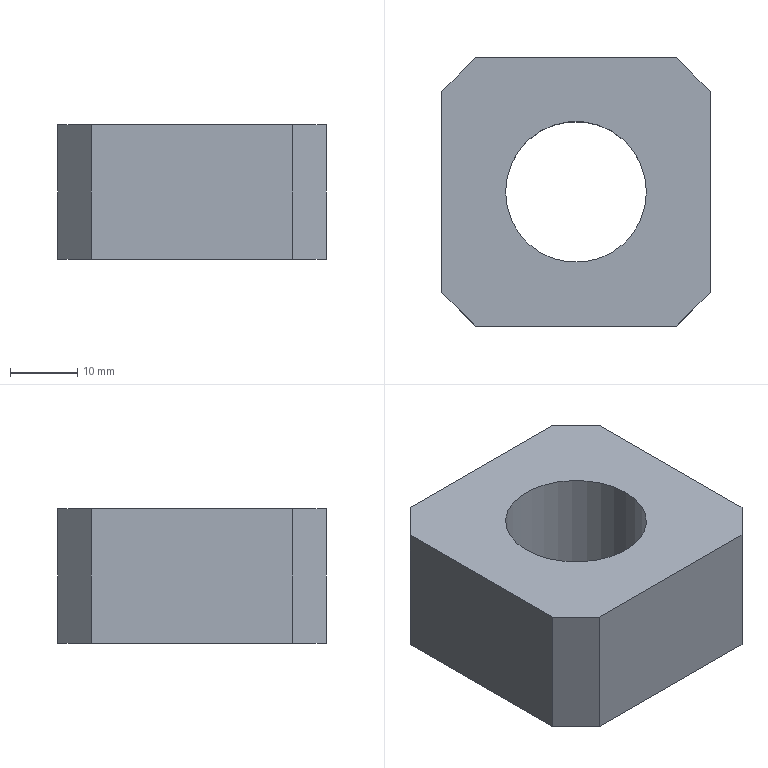Part | NX | 1 solid | 11 faces | box 40 x 40 x 20 mm | volume 24073 mm3 | plane 10 | cylinder 1 | commonest cylinder face diameters 21 x1
STEP:
#1=CARTESIAN_POINT('',(30.5,20.,20.));
#2=VERTEX_POINT('',#1);
#3=CARTESIAN_POINT('',(20.,20.,20.));
#4=DIRECTION('',(0.,0.,1.));
#5=DIRECTION('',(1.,0.,0.));
#6=AXIS2_PLACEMENT_3D('',#3,#4,#5);
#7=CIRCLE('',#6,10.5);
#8=EDGE_CURVE('',#2,#2,#7,.F.);
#9=ORIENTED_EDGE('',*,*,#8,.T.);
#10=EDGE_LOOP('',(#9));
#11=FACE_BOUND('',#10,.T.);
#12=CARTESIAN_POINT('',(35.,0.,20.));
#13=VERTEX_POINT('',#12);
#14=CARTESIAN_POINT('',(5.,0.,20.));
#15=VERTEX_POINT('',#14);
#16=CARTESIAN_POINT('',(20.,0.,20.));
#17=DIRECTION('',(-1.,0.,0.));
#18=VECTOR('',#17,1000.);
#19=LINE('',#16,#18);
#20=EDGE_CURVE('',#13,#15,#19,.T.);
#21=ORIENTED_EDGE('',*,*,#20,.F.);
#22=CARTESIAN_POINT('',(40.,5.,20.));
#23=VERTEX_POINT('',#22);
#24=CARTESIAN_POINT('',(37.5,2.5,20.));
#25=DIRECTION('',(-0.7071,-0.7071,0.));
#26=VECTOR('',#25,1000.);
#27=LINE('',#24,#26);
#28=EDGE_CURVE('',#13,#23,#27,.F.);
#29=ORIENTED_EDGE('',*,*,#28,.T.);
#30=CARTESIAN_POINT('',(40.,35.,20.));
#31=VERTEX_POINT('',#30);
#32=CARTESIAN_POINT('',(40.,20.,20.));
#33=DIRECTION('',(0.,-1.,0.));
#34=VECTOR('',#33,1000.);
#35=LINE('',#32,#34);
#36=EDGE_CURVE('',#31,#23,#35,.T.);
#37=ORIENTED_EDGE('',*,*,#36,.F.);
#38=CARTESIAN_POINT('',(35.,40.,20.));
#39=VERTEX_POINT('',#38);
#40=CARTESIAN_POINT('',(37.5,37.5,20.));
#41=DIRECTION('',(0.7071,-0.7071,0.));
#42=VECTOR('',#41,1000.);
#43=LINE('',#40,#42);
#44=EDGE_CURVE('',#31,#39,#43,.F.);
#45=ORIENTED_EDGE('',*,*,#44,.T.);
#46=CARTESIAN_POINT('',(5.,40.,20.));
#47=VERTEX_POINT('',#46);
#48=CARTESIAN_POINT('',(20.,40.,20.));
#49=DIRECTION('',(1.,0.,0.));
#50=VECTOR('',#49,1000.);
#51=LINE('',#48,#50);
#52=EDGE_CURVE('',#47,#39,#51,.T.);
#53=ORIENTED_EDGE('',*,*,#52,.F.);
#54=CARTESIAN_POINT('',(0.,35.,20.));
#55=VERTEX_POINT('',#54);
#56=CARTESIAN_POINT('',(2.5,37.5,20.));
#57=DIRECTION('',(0.7071,0.7071,0.));
#58=VECTOR('',#57,1000.);
#59=LINE('',#56,#58);
#60=EDGE_CURVE('',#47,#55,#59,.F.);
#61=ORIENTED_EDGE('',*,*,#60,.T.);
#62=CARTESIAN_POINT('',(0.,5.,20.));
#63=VERTEX_POINT('',#62);
#64=CARTESIAN_POINT('',(0.,20.,20.));
#65=DIRECTION('',(0.,1.,0.));
#66=VECTOR('',#65,1000.);
#67=LINE('',#64,#66);
#68=EDGE_CURVE('',#63,#55,#67,.T.);
#69=ORIENTED_EDGE('',*,*,#68,.F.);
#70=CARTESIAN_POINT('',(2.5,2.5,20.));
#71=DIRECTION('',(-0.7071,0.7071,0.));
#72=VECTOR('',#71,1000.);
#73=LINE('',#70,#72);
#74=EDGE_CURVE('',#63,#15,#73,.F.);
#75=ORIENTED_EDGE('',*,*,#74,.T.);
#76=EDGE_LOOP('',(#21,#29,#37,#45,#53,#61,#69,#75));
#77=FACE_BOUND('',#76,.T.);
#78=CARTESIAN_POINT('',(20.,20.,20.));
#79=DIRECTION('',(0.,0.,1.));
#80=DIRECTION('',(1.,0.,0.));
#81=AXIS2_PLACEMENT_3D('',#78,#79,#80);
#82=PLANE('',#81);
#83=ADVANCED_FACE('',(#11,#77),#82,.T.);
#84=CARTESIAN_POINT('',(5.,0.,0.));
#85=VERTEX_POINT('',#84);
#86=CARTESIAN_POINT('',(35.,0.,0.));
#87=VERTEX_POINT('',#86);
#88=CARTESIAN_POINT('',(20.,0.,0.));
#89=DIRECTION('',(1.,0.,0.));
#90=VECTOR('',#89,1000.);
#91=LINE('',#88,#90);
#92=EDGE_CURVE('',#85,#87,#91,.T.);
#93=ORIENTED_EDGE('',*,*,#92,.T.);
#94=CARTESIAN_POINT('',(35.,0.,0.));
#95=DIRECTION('',(0.,0.,1.));
#96=VECTOR('',#95,1000.);
#97=LINE('',#94,#96);
#98=EDGE_CURVE('',#87,#13,#97,.T.);
#99=ORIENTED_EDGE('',*,*,#98,.T.);
#100=ORIENTED_EDGE('',*,*,#20,.T.);
#101=CARTESIAN_POINT('',(5.,0.,0.));
#102=DIRECTION('',(0.,0.,-1.));
#103=VECTOR('',#102,1000.);
#104=LINE('',#101,#103);
#105=EDGE_CURVE('',#15,#85,#104,.T.);
#106=ORIENTED_EDGE('',*,*,#105,.T.);
#107=EDGE_LOOP('',(#93,#99,#100,#106));
#108=FACE_BOUND('',#107,.T.);
#109=CARTESIAN_POINT('',(20.,0.,0.));
#110=DIRECTION('',(0.,-1.,0.));
#111=DIRECTION('',(0.,0.,-1.));
#112=AXIS2_PLACEMENT_3D('',#109,#110,#111);
#113=PLANE('',#112);
#114=ADVANCED_FACE('',(#108),#113,.T.);
#115=ORIENTED_EDGE('',*,*,#68,.T.);
#116=CARTESIAN_POINT('',(0.,35.,0.));
#117=VERTEX_POINT('',#116);
#118=CARTESIAN_POINT('',(0.,35.,0.));
#119=DIRECTION('',(0.,0.,-1.));
#120=VECTOR('',#119,1000.);
#121=LINE('',#118,#120);
#122=EDGE_CURVE('',#55,#117,#121,.T.);
#123=ORIENTED_EDGE('',*,*,#122,.T.);
#124=CARTESIAN_POINT('',(0.,5.,0.));
#125=VERTEX_POINT('',#124);
#126=CARTESIAN_POINT('',(0.,20.,0.));
#127=DIRECTION('',(0.,-1.,0.));
#128=VECTOR('',#127,1000.);
#129=LINE('',#126,#128);
#130=EDGE_CURVE('',#117,#125,#129,.T.);
#131=ORIENTED_EDGE('',*,*,#130,.T.);
#132=CARTESIAN_POINT('',(0.,5.,0.));
#133=DIRECTION('',(0.,0.,1.));
#134=VECTOR('',#133,1000.);
#135=LINE('',#132,#134);
#136=EDGE_CURVE('',#125,#63,#135,.T.);
#137=ORIENTED_EDGE('',*,*,#136,.T.);
#138=EDGE_LOOP('',(#115,#123,#131,#137));
#139=FACE_BOUND('',#138,.T.);
#140=CARTESIAN_POINT('',(0.,20.,0.));
#141=DIRECTION('',(-1.,0.,0.));
#142=DIRECTION('',(0.,0.,1.));
#143=AXIS2_PLACEMENT_3D('',#140,#141,#142);
#144=PLANE('',#143);
#145=ADVANCED_FACE('',(#139),#144,.T.);
#146=ORIENTED_EDGE('',*,*,#52,.T.);
#147=CARTESIAN_POINT('',(35.,40.,0.));
#148=VERTEX_POINT('',#147);
#149=CARTESIAN_POINT('',(35.,40.,0.));
#150=DIRECTION('',(0.,0.,-1.));
#151=VECTOR('',#150,1000.);
#152=LINE('',#149,#151);
#153=EDGE_CURVE('',#39,#148,#152,.T.);
#154=ORIENTED_EDGE('',*,*,#153,.T.);
#155=CARTESIAN_POINT('',(5.,40.,0.));
#156=VERTEX_POINT('',#155);
#157=CARTESIAN_POINT('',(20.,40.,0.));
#158=DIRECTION('',(-1.,0.,0.));
#159=VECTOR('',#158,1000.);
#160=LINE('',#157,#159);
#161=EDGE_CURVE('',#148,#156,#160,.T.);
#162=ORIENTED_EDGE('',*,*,#161,.T.);
#163=CARTESIAN_POINT('',(5.,40.,0.));
#164=DIRECTION('',(0.,0.,1.));
#165=VECTOR('',#164,1000.);
#166=LINE('',#163,#165);
#167=EDGE_CURVE('',#156,#47,#166,.T.);
#168=ORIENTED_EDGE('',*,*,#167,.T.);
#169=EDGE_LOOP('',(#146,#154,#162,#168));
#170=FACE_BOUND('',#169,.T.);
#171=CARTESIAN_POINT('',(20.,40.,0.));
#172=DIRECTION('',(0.,1.,0.));
#173=DIRECTION('',(0.,0.,1.));
#174=AXIS2_PLACEMENT_3D('',#171,#172,#173);
#175=PLANE('',#174);
#176=ADVANCED_FACE('',(#170),#175,.T.);
#177=CARTESIAN_POINT('',(9.5,20.,0.));
#178=VERTEX_POINT('',#177);
#179=CARTESIAN_POINT('',(20.,20.,0.));
#180=DIRECTION('',(0.,0.,-1.));
#181=DIRECTION('',(-1.,0.,0.));
#182=AXIS2_PLACEMENT_3D('',#179,#180,#181);
#183=CIRCLE('',#182,10.5);
#184=EDGE_CURVE('',#178,#178,#183,.T.);
#185=ORIENTED_EDGE('',*,*,#184,.F.);
#186=EDGE_LOOP('',(#185));
#187=FACE_BOUND('',#186,.T.);
#188=CARTESIAN_POINT('',(40.,5.,0.));
#189=VERTEX_POINT('',#188);
#190=CARTESIAN_POINT('',(40.,35.,0.));
#191=VERTEX_POINT('',#190);
#192=CARTESIAN_POINT('',(40.,20.,0.));
#193=DIRECTION('',(0.,1.,0.));
#194=VECTOR('',#193,1000.);
#195=LINE('',#192,#194);
#196=EDGE_CURVE('',#189,#191,#195,.T.);
#197=ORIENTED_EDGE('',*,*,#196,.F.);
#198=CARTESIAN_POINT('',(37.5,2.5,0.));
#199=DIRECTION('',(0.7071,0.7071,0.));
#200=VECTOR('',#199,1000.);
#201=LINE('',#198,#200);
#202=EDGE_CURVE('',#189,#87,#201,.F.);
#203=ORIENTED_EDGE('',*,*,#202,.T.);
#204=ORIENTED_EDGE('',*,*,#92,.F.);
#205=CARTESIAN_POINT('',(2.5,2.5,0.));
#206=DIRECTION('',(0.7071,-0.7071,0.));
#207=VECTOR('',#206,1000.);
#208=LINE('',#205,#207);
#209=EDGE_CURVE('',#85,#125,#208,.F.);
#210=ORIENTED_EDGE('',*,*,#209,.T.);
#211=ORIENTED_EDGE('',*,*,#130,.F.);
#212=CARTESIAN_POINT('',(2.5,37.5,0.));
#213=DIRECTION('',(-0.7071,-0.7071,0.));
#214=VECTOR('',#213,1000.);
#215=LINE('',#212,#214);
#216=EDGE_CURVE('',#117,#156,#215,.F.);
#217=ORIENTED_EDGE('',*,*,#216,.T.);
#218=ORIENTED_EDGE('',*,*,#161,.F.);
#219=CARTESIAN_POINT('',(37.5,37.5,0.));
#220=DIRECTION('',(-0.7071,0.7071,0.));
#221=VECTOR('',#220,1000.);
#222=LINE('',#219,#221);
#223=EDGE_CURVE('',#148,#191,#222,.F.);
#224=ORIENTED_EDGE('',*,*,#223,.T.);
#225=EDGE_LOOP('',(#197,#203,#204,#210,#211,#217,#218,#224));
#226=FACE_BOUND('',#225,.T.);
#227=CARTESIAN_POINT('',(20.,20.,0.));
#228=DIRECTION('',(0.,0.,-1.));
#229=DIRECTION('',(-1.,0.,0.));
#230=AXIS2_PLACEMENT_3D('',#227,#228,#229);
#231=PLANE('',#230);
#232=ADVANCED_FACE('',(#187,#226),#231,.T.);
#233=ORIENTED_EDGE('',*,*,#36,.T.);
#234=CARTESIAN_POINT('',(40.,5.,0.));
#235=DIRECTION('',(0.,0.,-1.));
#236=VECTOR('',#235,1000.);
#237=LINE('',#234,#236);
#238=EDGE_CURVE('',#23,#189,#237,.T.);
#239=ORIENTED_EDGE('',*,*,#238,.T.);
#240=ORIENTED_EDGE('',*,*,#196,.T.);
#241=CARTESIAN_POINT('',(40.,35.,0.));
#242=DIRECTION('',(0.,0.,1.));
#243=VECTOR('',#242,1000.);
#244=LINE('',#241,#243);
#245=EDGE_CURVE('',#191,#31,#244,.T.);
#246=ORIENTED_EDGE('',*,*,#245,.T.);
#247=EDGE_LOOP('',(#233,#239,#240,#246));
#248=FACE_BOUND('',#247,.T.);
#249=CARTESIAN_POINT('',(40.,20.,0.));
#250=DIRECTION('',(1.,0.,0.));
#251=DIRECTION('',(0.,0.,-1.));
#252=AXIS2_PLACEMENT_3D('',#249,#250,#251);
#253=PLANE('',#252);
#254=ADVANCED_FACE('',(#248),#253,.T.);
#255=ORIENTED_EDGE('',*,*,#202,.F.);
#256=ORIENTED_EDGE('',*,*,#238,.F.);
#257=ORIENTED_EDGE('',*,*,#28,.F.);
#258=ORIENTED_EDGE('',*,*,#98,.F.);
#259=EDGE_LOOP('',(#255,#256,#257,#258));
#260=FACE_BOUND('',#259,.T.);
#261=CARTESIAN_POINT('',(35.,0.,0.));
#262=DIRECTION('',(-0.7071,0.7071,0.));
#263=DIRECTION('',(0.,0.,1.));
#264=AXIS2_PLACEMENT_3D('',#261,#262,#263);
#265=PLANE('',#264);
#266=ADVANCED_FACE('',(#260),#265,.F.);
#267=ORIENTED_EDGE('',*,*,#223,.F.);
#268=ORIENTED_EDGE('',*,*,#153,.F.);
#269=ORIENTED_EDGE('',*,*,#44,.F.);
#270=ORIENTED_EDGE('',*,*,#245,.F.);
#271=EDGE_LOOP('',(#267,#268,#269,#270));
#272=FACE_BOUND('',#271,.T.);
#273=CARTESIAN_POINT('',(40.,35.,0.));
#274=DIRECTION('',(-0.7071,-0.7071,0.));
#275=DIRECTION('',(0.,0.,1.));
#276=AXIS2_PLACEMENT_3D('',#273,#274,#275);
#277=PLANE('',#276);
#278=ADVANCED_FACE('',(#272),#277,.F.);
#279=ORIENTED_EDGE('',*,*,#216,.F.);
#280=ORIENTED_EDGE('',*,*,#122,.F.);
#281=ORIENTED_EDGE('',*,*,#60,.F.);
#282=ORIENTED_EDGE('',*,*,#167,.F.);
#283=EDGE_LOOP('',(#279,#280,#281,#282));
#284=FACE_BOUND('',#283,.T.);
#285=CARTESIAN_POINT('',(5.,40.,0.));
#286=DIRECTION('',(0.7071,-0.7071,0.));
#287=DIRECTION('',(0.,0.,1.));
#288=AXIS2_PLACEMENT_3D('',#285,#286,#287);
#289=PLANE('',#288);
#290=ADVANCED_FACE('',(#284),#289,.F.);
#291=ORIENTED_EDGE('',*,*,#209,.F.);
#292=ORIENTED_EDGE('',*,*,#105,.F.);
#293=ORIENTED_EDGE('',*,*,#74,.F.);
#294=ORIENTED_EDGE('',*,*,#136,.F.);
#295=EDGE_LOOP('',(#291,#292,#293,#294));
#296=FACE_BOUND('',#295,.T.);
#297=CARTESIAN_POINT('',(0.,5.,0.));
#298=DIRECTION('',(0.7071,0.7071,0.));
#299=DIRECTION('',(0.,0.,1.));
#300=AXIS2_PLACEMENT_3D('',#297,#298,#299);
#301=PLANE('',#300);
#302=ADVANCED_FACE('',(#296),#301,.F.);
#303=ORIENTED_EDGE('',*,*,#184,.T.);
#304=EDGE_LOOP('',(#303));
#305=FACE_BOUND('',#304,.T.);
#306=ORIENTED_EDGE('',*,*,#8,.F.);
#307=EDGE_LOOP('',(#306));
#308=FACE_BOUND('',#307,.T.);
#309=CARTESIAN_POINT('',(20.,20.,20.));
#310=DIRECTION('',(0.,0.,-1.));
#311=DIRECTION('',(1.,0.,0.));
#312=AXIS2_PLACEMENT_3D('',#309,#310,#311);
#313=CYLINDRICAL_SURFACE('',#312,10.5);
#314=ADVANCED_FACE('',(#305,#308),#313,.F.);
#315=CLOSED_SHELL('',(#83,#114,#145,#176,#232,#254,#266,#278,#290,#302,#314));
#316=MANIFOLD_SOLID_BREP('',#315);
#317=(LENGTH_UNIT()NAMED_UNIT(*)SI_UNIT(.MILLI.,.METRE.));
#318=UNCERTAINTY_MEASURE_WITH_UNIT(LENGTH_MEASURE(0.00001),#317,'','');
#319=(NAMED_UNIT(*)PLANE_ANGLE_UNIT()SI_UNIT($,.RADIAN.));
#320=(NAMED_UNIT(*)SI_UNIT($,.STERADIAN.)SOLID_ANGLE_UNIT());
#321=(GEOMETRIC_REPRESENTATION_CONTEXT(3)GLOBAL_UNCERTAINTY_ASSIGNED_CONTEXT((#318))GLOBAL_UNIT_ASSIGNED_CONTEXT((#317,#319,#320))REPRESENTATION_CONTEXT('',''));
#322=ADVANCED_BREP_SHAPE_REPRESENTATION('',(#316),#321);